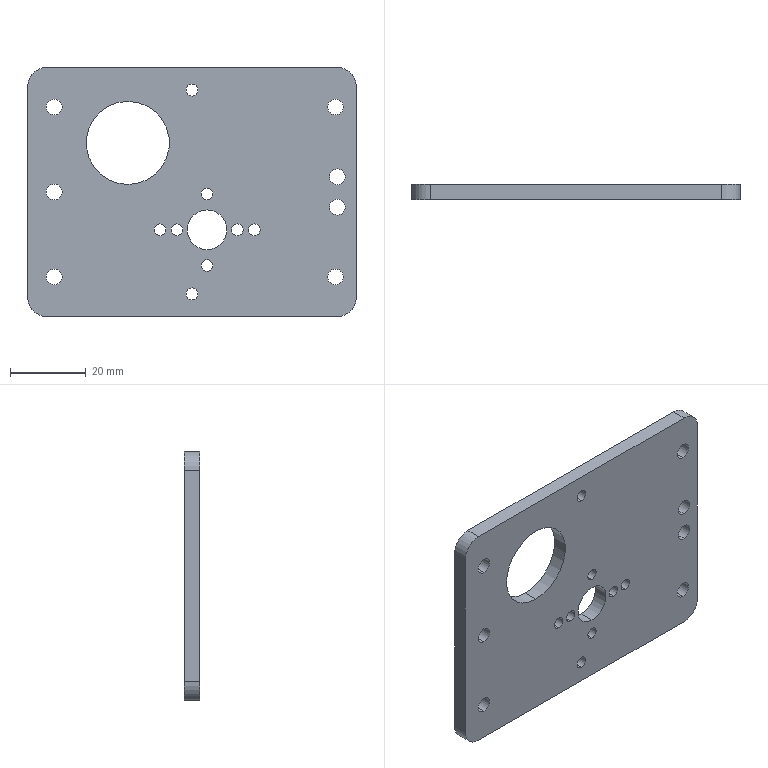Part | SolidWorks | features BaseBody 1 | 1 solid | 44 faces | box 87 x 4 x 66 mm | volume 20382 mm3 | cylinder 38 | plane 6 | commonest cylinder face diameters 4.2 x14 3.1 x12 3.2 x4 10 x4 10.5 x2 22 x2
STEP:
#1=CARTESIAN_POINT('',(38.5,4.,6.1));
#2=VERTEX_POINT('',#1);
#3=CARTESIAN_POINT('',(38.5,4.,1.9));
#4=VERTEX_POINT('',#3);
#5=CARTESIAN_POINT('',(38.5,4.,4.));
#6=DIRECTION('',(0.,-1.,0.));
#7=DIRECTION('',(0.,0.,-1.));
#8=AXIS2_PLACEMENT_3D('',#5,#6,#7);
#9=CIRCLE('',#8,2.1);
#10=EDGE_CURVE('',#2,#4,#9,.T.);
#11=ORIENTED_EDGE('',*,*,#10,.F.);
#12=CARTESIAN_POINT('',(38.5,0.,6.1));
#13=VERTEX_POINT('',#12);
#14=CARTESIAN_POINT('',(38.5,4.,6.1));
#15=DIRECTION('',(0.,-1.,0.));
#16=VECTOR('',#15,1000.);
#17=LINE('',#14,#16);
#18=EDGE_CURVE('',#2,#13,#17,.T.);
#19=ORIENTED_EDGE('',*,*,#18,.T.);
#20=CARTESIAN_POINT('',(38.5,0.,1.9));
#21=VERTEX_POINT('',#20);
#22=CARTESIAN_POINT('',(38.5,0.,4.));
#23=DIRECTION('',(0.,-1.,0.));
#24=DIRECTION('',(0.,0.,-1.));
#25=AXIS2_PLACEMENT_3D('',#22,#23,#24);
#26=CIRCLE('',#25,2.1);
#27=EDGE_CURVE('',#13,#21,#26,.T.);
#28=ORIENTED_EDGE('',*,*,#27,.T.);
#29=CARTESIAN_POINT('',(38.5,4.,1.9));
#30=DIRECTION('',(0.,-1.,0.));
#31=VECTOR('',#30,1000.);
#32=LINE('',#29,#31);
#33=EDGE_CURVE('',#4,#21,#32,.T.);
#34=ORIENTED_EDGE('',*,*,#33,.F.);
#35=EDGE_LOOP('',(#11,#19,#28,#34));
#36=FACE_OUTER_BOUND('',#35,.T.);
#37=CARTESIAN_POINT('',(38.5,4.,4.));
#38=DIRECTION('',(0.,-1.,0.));
#39=DIRECTION('',(0.,0.,-1.));
#40=AXIS2_PLACEMENT_3D('',#37,#38,#39);
#41=CYLINDRICAL_SURFACE('',#40,2.1);
#42=ADVANCED_FACE('',(#36),#41,.F.);
#43=CARTESIAN_POINT('',(38.5,4.,-1.9));
#44=VERTEX_POINT('',#43);
#45=CARTESIAN_POINT('',(38.5,4.,-6.1));
#46=VERTEX_POINT('',#45);
#47=CARTESIAN_POINT('',(38.5,4.,-4.));
#48=DIRECTION('',(0.,-1.,0.));
#49=DIRECTION('',(0.,0.,-1.));
#50=AXIS2_PLACEMENT_3D('',#47,#48,#49);
#51=CIRCLE('',#50,2.1);
#52=EDGE_CURVE('',#44,#46,#51,.T.);
#53=ORIENTED_EDGE('',*,*,#52,.F.);
#54=CARTESIAN_POINT('',(38.5,0.,-1.9));
#55=VERTEX_POINT('',#54);
#56=CARTESIAN_POINT('',(38.5,4.,-1.9));
#57=DIRECTION('',(0.,-1.,0.));
#58=VECTOR('',#57,1000.);
#59=LINE('',#56,#58);
#60=EDGE_CURVE('',#44,#55,#59,.T.);
#61=ORIENTED_EDGE('',*,*,#60,.T.);
#62=CARTESIAN_POINT('',(38.5,0.,-6.1));
#63=VERTEX_POINT('',#62);
#64=CARTESIAN_POINT('',(38.5,0.,-4.));
#65=DIRECTION('',(0.,-1.,0.));
#66=DIRECTION('',(0.,0.,-1.));
#67=AXIS2_PLACEMENT_3D('',#64,#65,#66);
#68=CIRCLE('',#67,2.1);
#69=EDGE_CURVE('',#55,#63,#68,.T.);
#70=ORIENTED_EDGE('',*,*,#69,.T.);
#71=CARTESIAN_POINT('',(38.5,4.,-6.1));
#72=DIRECTION('',(0.,-1.,0.));
#73=VECTOR('',#72,1000.);
#74=LINE('',#71,#73);
#75=EDGE_CURVE('',#46,#63,#74,.T.);
#76=ORIENTED_EDGE('',*,*,#75,.F.);
#77=EDGE_LOOP('',(#53,#61,#70,#76));
#78=FACE_OUTER_BOUND('',#77,.T.);
#79=CARTESIAN_POINT('',(38.5,4.,-4.));
#80=DIRECTION('',(0.,-1.,0.));
#81=DIRECTION('',(0.,0.,-1.));
#82=AXIS2_PLACEMENT_3D('',#79,#80,#81);
#83=CYLINDRICAL_SURFACE('',#82,2.1);
#84=ADVANCED_FACE('',(#78),#83,.F.);
#85=CARTESIAN_POINT('',(0.,4.,28.6));
#86=VERTEX_POINT('',#85);
#87=CARTESIAN_POINT('',(0.,4.,25.4));
#88=VERTEX_POINT('',#87);
#89=CARTESIAN_POINT('',(0.,4.,27.));
#90=DIRECTION('',(0.,-1.,0.));
#91=DIRECTION('',(0.,0.,-1.));
#92=AXIS2_PLACEMENT_3D('',#89,#90,#91);
#93=CIRCLE('',#92,1.6);
#94=EDGE_CURVE('',#86,#88,#93,.T.);
#95=ORIENTED_EDGE('',*,*,#94,.F.);
#96=CARTESIAN_POINT('',(0.,0.,28.6));
#97=VERTEX_POINT('',#96);
#98=CARTESIAN_POINT('',(0.,4.,28.6));
#99=DIRECTION('',(0.,-1.,0.));
#100=VECTOR('',#99,1000.);
#101=LINE('',#98,#100);
#102=EDGE_CURVE('',#86,#97,#101,.T.);
#103=ORIENTED_EDGE('',*,*,#102,.T.);
#104=CARTESIAN_POINT('',(0.,0.,25.4));
#105=VERTEX_POINT('',#104);
#106=CARTESIAN_POINT('',(0.,0.,27.));
#107=DIRECTION('',(0.,-1.,0.));
#108=DIRECTION('',(0.,0.,-1.));
#109=AXIS2_PLACEMENT_3D('',#106,#107,#108);
#110=CIRCLE('',#109,1.6);
#111=EDGE_CURVE('',#97,#105,#110,.T.);
#112=ORIENTED_EDGE('',*,*,#111,.T.);
#113=CARTESIAN_POINT('',(0.,4.,25.4));
#114=DIRECTION('',(0.,-1.,0.));
#115=VECTOR('',#114,1000.);
#116=LINE('',#113,#115);
#117=EDGE_CURVE('',#88,#105,#116,.T.);
#118=ORIENTED_EDGE('',*,*,#117,.F.);
#119=EDGE_LOOP('',(#95,#103,#112,#118));
#120=FACE_OUTER_BOUND('',#119,.T.);
#121=CARTESIAN_POINT('',(0.,4.,27.));
#122=DIRECTION('',(0.,-1.,0.));
#123=DIRECTION('',(0.,0.,-1.));
#124=AXIS2_PLACEMENT_3D('',#121,#122,#123);
#125=CYLINDRICAL_SURFACE('',#124,1.6);
#126=ADVANCED_FACE('',(#120),#125,.F.);
#127=CARTESIAN_POINT('',(38.,4.,-20.4));
#128=VERTEX_POINT('',#127);
#129=CARTESIAN_POINT('',(38.,4.,-24.6));
#130=VERTEX_POINT('',#129);
#131=CARTESIAN_POINT('',(38.,4.,-22.5));
#132=DIRECTION('',(0.,-1.,0.));
#133=DIRECTION('',(0.,0.,-1.));
#134=AXIS2_PLACEMENT_3D('',#131,#132,#133);
#135=CIRCLE('',#134,2.1);
#136=EDGE_CURVE('',#128,#130,#135,.T.);
#137=ORIENTED_EDGE('',*,*,#136,.F.);
#138=CARTESIAN_POINT('',(38.,0.,-20.4));
#139=VERTEX_POINT('',#138);
#140=CARTESIAN_POINT('',(38.,4.,-20.4));
#141=DIRECTION('',(0.,-1.,0.));
#142=VECTOR('',#141,1000.);
#143=LINE('',#140,#142);
#144=EDGE_CURVE('',#128,#139,#143,.T.);
#145=ORIENTED_EDGE('',*,*,#144,.T.);
#146=CARTESIAN_POINT('',(38.,0.,-24.6));
#147=VERTEX_POINT('',#146);
#148=CARTESIAN_POINT('',(38.,0.,-22.5));
#149=DIRECTION('',(0.,-1.,0.));
#150=DIRECTION('',(0.,0.,-1.));
#151=AXIS2_PLACEMENT_3D('',#148,#149,#150);
#152=CIRCLE('',#151,2.1);
#153=EDGE_CURVE('',#139,#147,#152,.T.);
#154=ORIENTED_EDGE('',*,*,#153,.T.);
#155=CARTESIAN_POINT('',(38.,4.,-24.6));
#156=DIRECTION('',(0.,-1.,0.));
#157=VECTOR('',#156,1000.);
#158=LINE('',#155,#157);
#159=EDGE_CURVE('',#130,#147,#158,.T.);
#160=ORIENTED_EDGE('',*,*,#159,.F.);
#161=EDGE_LOOP('',(#137,#145,#154,#160));
#162=FACE_OUTER_BOUND('',#161,.T.);
#163=CARTESIAN_POINT('',(38.,4.,-22.5));
#164=DIRECTION('',(0.,-1.,0.));
#165=DIRECTION('',(0.,0.,-1.));
#166=AXIS2_PLACEMENT_3D('',#163,#164,#165);
#167=CYLINDRICAL_SURFACE('',#166,2.1);
#168=ADVANCED_FACE('',(#162),#167,.F.);
#169=CARTESIAN_POINT('',(38.,4.,24.6));
#170=VERTEX_POINT('',#169);
#171=CARTESIAN_POINT('',(38.,4.,20.4));
#172=VERTEX_POINT('',#171);
#173=CARTESIAN_POINT('',(38.,4.,22.5));
#174=DIRECTION('',(0.,-1.,0.));
#175=DIRECTION('',(0.,0.,-1.));
#176=AXIS2_PLACEMENT_3D('',#173,#174,#175);
#177=CIRCLE('',#176,2.1);
#178=EDGE_CURVE('',#170,#172,#177,.T.);
#179=ORIENTED_EDGE('',*,*,#178,.F.);
#180=CARTESIAN_POINT('',(38.,0.,24.6));
#181=VERTEX_POINT('',#180);
#182=CARTESIAN_POINT('',(38.,4.,24.6));
#183=DIRECTION('',(0.,-1.,0.));
#184=VECTOR('',#183,1000.);
#185=LINE('',#182,#184);
#186=EDGE_CURVE('',#170,#181,#185,.T.);
#187=ORIENTED_EDGE('',*,*,#186,.T.);
#188=CARTESIAN_POINT('',(38.,0.,20.4));
#189=VERTEX_POINT('',#188);
#190=CARTESIAN_POINT('',(38.,0.,22.5));
#191=DIRECTION('',(0.,-1.,0.));
#192=DIRECTION('',(0.,0.,-1.));
#193=AXIS2_PLACEMENT_3D('',#190,#191,#192);
#194=CIRCLE('',#193,2.1);
#195=EDGE_CURVE('',#181,#189,#194,.T.);
#196=ORIENTED_EDGE('',*,*,#195,.T.);
#197=CARTESIAN_POINT('',(38.,4.,20.4));
#198=DIRECTION('',(0.,-1.,0.));
#199=VECTOR('',#198,1000.);
#200=LINE('',#197,#199);
#201=EDGE_CURVE('',#172,#189,#200,.T.);
#202=ORIENTED_EDGE('',*,*,#201,.F.);
#203=EDGE_LOOP('',(#179,#187,#196,#202));
#204=FACE_OUTER_BOUND('',#203,.T.);
#205=CARTESIAN_POINT('',(38.,4.,22.5));
#206=DIRECTION('',(0.,-1.,0.));
#207=DIRECTION('',(0.,0.,-1.));
#208=AXIS2_PLACEMENT_3D('',#205,#206,#207);
#209=CYLINDRICAL_SURFACE('',#208,2.1);
#210=ADVANCED_FACE('',(#204),#209,.F.);
#211=CARTESIAN_POINT('',(-36.5,4.,24.6));
#212=VERTEX_POINT('',#211);
#213=CARTESIAN_POINT('',(-36.5,4.,20.4));
#214=VERTEX_POINT('',#213);
#215=CARTESIAN_POINT('',(-36.5,4.,22.5));
#216=DIRECTION('',(0.,-1.,0.));
#217=DIRECTION('',(0.,0.,-1.));
#218=AXIS2_PLACEMENT_3D('',#215,#216,#217);
#219=CIRCLE('',#218,2.1);
#220=EDGE_CURVE('',#212,#214,#219,.T.);
#221=ORIENTED_EDGE('',*,*,#220,.F.);
#222=CARTESIAN_POINT('',(-36.5,0.,24.6));
#223=VERTEX_POINT('',#222);
#224=CARTESIAN_POINT('',(-36.5,4.,24.6));
#225=DIRECTION('',(0.,-1.,0.));
#226=VECTOR('',#225,1000.);
#227=LINE('',#224,#226);
#228=EDGE_CURVE('',#212,#223,#227,.T.);
#229=ORIENTED_EDGE('',*,*,#228,.T.);
#230=CARTESIAN_POINT('',(-36.5,0.,20.4));
#231=VERTEX_POINT('',#230);
#232=CARTESIAN_POINT('',(-36.5,0.,22.5));
#233=DIRECTION('',(0.,-1.,0.));
#234=DIRECTION('',(0.,0.,-1.));
#235=AXIS2_PLACEMENT_3D('',#232,#233,#234);
#236=CIRCLE('',#235,2.1);
#237=EDGE_CURVE('',#223,#231,#236,.T.);
#238=ORIENTED_EDGE('',*,*,#237,.T.);
#239=CARTESIAN_POINT('',(-36.5,4.,20.4));
#240=DIRECTION('',(0.,-1.,0.));
#241=VECTOR('',#240,1000.);
#242=LINE('',#239,#241);
#243=EDGE_CURVE('',#214,#231,#242,.T.);
#244=ORIENTED_EDGE('',*,*,#243,.F.);
#245=EDGE_LOOP('',(#221,#229,#238,#244));
#246=FACE_OUTER_BOUND('',#245,.T.);
#247=CARTESIAN_POINT('',(-36.5,4.,22.5));
#248=DIRECTION('',(0.,-1.,0.));
#249=DIRECTION('',(0.,0.,-1.));
#250=AXIS2_PLACEMENT_3D('',#247,#248,#249);
#251=CYLINDRICAL_SURFACE('',#250,2.1);
#252=ADVANCED_FACE('',(#246),#251,.F.);
#253=CARTESIAN_POINT('',(-36.5,4.,2.1));
#254=VERTEX_POINT('',#253);
#255=CARTESIAN_POINT('',(-36.5,4.,-2.1));
#256=VERTEX_POINT('',#255);
#257=CARTESIAN_POINT('',(-36.5,4.,0.));
#258=DIRECTION('',(0.,-1.,0.));
#259=DIRECTION('',(0.,0.,-1.));
#260=AXIS2_PLACEMENT_3D('',#257,#258,#259);
#261=CIRCLE('',#260,2.1);
#262=EDGE_CURVE('',#254,#256,#261,.T.);
#263=ORIENTED_EDGE('',*,*,#262,.F.);
#264=CARTESIAN_POINT('',(-36.5,0.,2.1));
#265=VERTEX_POINT('',#264);
#266=CARTESIAN_POINT('',(-36.5,4.,2.1));
#267=DIRECTION('',(0.,-1.,0.));
#268=VECTOR('',#267,1000.);
#269=LINE('',#266,#268);
#270=EDGE_CURVE('',#254,#265,#269,.T.);
#271=ORIENTED_EDGE('',*,*,#270,.T.);
#272=CARTESIAN_POINT('',(-36.5,0.,-2.1));
#273=VERTEX_POINT('',#272);
#274=CARTESIAN_POINT('',(-36.5,0.,0.));
#275=DIRECTION('',(0.,-1.,0.));
#276=DIRECTION('',(0.,0.,-1.));
#277=AXIS2_PLACEMENT_3D('',#274,#275,#276);
#278=CIRCLE('',#277,2.1);
#279=EDGE_CURVE('',#265,#273,#278,.T.);
#280=ORIENTED_EDGE('',*,*,#279,.T.);
#281=CARTESIAN_POINT('',(-36.5,4.,-2.1));
#282=DIRECTION('',(0.,-1.,0.));
#283=VECTOR('',#282,1000.);
#284=LINE('',#281,#283);
#285=EDGE_CURVE('',#256,#273,#284,.T.);
#286=ORIENTED_EDGE('',*,*,#285,.F.);
#287=EDGE_LOOP('',(#263,#271,#280,#286));
#288=FACE_OUTER_BOUND('',#287,.T.);
#289=CARTESIAN_POINT('',(-36.5,4.,0.));
#290=DIRECTION('',(0.,-1.,0.));
#291=DIRECTION('',(0.,0.,-1.));
#292=AXIS2_PLACEMENT_3D('',#289,#290,#291);
#293=CYLINDRICAL_SURFACE('',#292,2.1);
#294=ADVANCED_FACE('',(#288),#293,.F.);
#295=CARTESIAN_POINT('',(-36.5,4.,-20.4));
#296=VERTEX_POINT('',#295);
#297=CARTESIAN_POINT('',(-36.5,4.,-24.6));
#298=VERTEX_POINT('',#297);
#299=CARTESIAN_POINT('',(-36.5,4.,-22.5));
#300=DIRECTION('',(0.,-1.,0.));
#301=DIRECTION('',(0.,0.,-1.));
#302=AXIS2_PLACEMENT_3D('',#299,#300,#301);
#303=CIRCLE('',#302,2.1);
#304=EDGE_CURVE('',#296,#298,#303,.T.);
#305=ORIENTED_EDGE('',*,*,#304,.F.);
#306=CARTESIAN_POINT('',(-36.5,0.,-20.4));
#307=VERTEX_POINT('',#306);
#308=CARTESIAN_POINT('',(-36.5,4.,-20.4));
#309=DIRECTION('',(0.,-1.,0.));
#310=VECTOR('',#309,1000.);
#311=LINE('',#308,#310);
#312=EDGE_CURVE('',#296,#307,#311,.T.);
#313=ORIENTED_EDGE('',*,*,#312,.T.);
#314=CARTESIAN_POINT('',(-36.5,0.,-24.6));
#315=VERTEX_POINT('',#314);
#316=CARTESIAN_POINT('',(-36.5,0.,-22.5));
#317=DIRECTION('',(0.,-1.,0.));
#318=DIRECTION('',(0.,0.,-1.));
#319=AXIS2_PLACEMENT_3D('',#316,#317,#318);
#320=CIRCLE('',#319,2.1);
#321=EDGE_CURVE('',#307,#315,#320,.T.);
#322=ORIENTED_EDGE('',*,*,#321,.T.);
#323=CARTESIAN_POINT('',(-36.5,4.,-24.6));
#324=DIRECTION('',(0.,-1.,0.));
#325=VECTOR('',#324,1000.);
#326=LINE('',#323,#325);
#327=EDGE_CURVE('',#298,#315,#326,.T.);
#328=ORIENTED_EDGE('',*,*,#327,.F.);
#329=EDGE_LOOP('',(#305,#313,#322,#328));
#330=FACE_OUTER_BOUND('',#329,.T.);
#331=CARTESIAN_POINT('',(-36.5,4.,-22.5));
#332=DIRECTION('',(0.,-1.,0.));
#333=DIRECTION('',(0.,0.,-1.));
#334=AXIS2_PLACEMENT_3D('',#331,#332,#333);
#335=CYLINDRICAL_SURFACE('',#334,2.1);
#336=ADVANCED_FACE('',(#330),#335,.F.);
#337=CARTESIAN_POINT('',(0.,4.,-25.4));
#338=VERTEX_POINT('',#337);
#339=CARTESIAN_POINT('',(0.,4.,-28.6));
#340=VERTEX_POINT('',#339);
#341=CARTESIAN_POINT('',(0.,4.,-27.));
#342=DIRECTION('',(0.,-1.,0.));
#343=DIRECTION('',(0.,0.,-1.));
#344=AXIS2_PLACEMENT_3D('',#341,#342,#343);
#345=CIRCLE('',#344,1.6);
#346=EDGE_CURVE('',#338,#340,#345,.T.);
#347=ORIENTED_EDGE('',*,*,#346,.F.);
#348=CARTESIAN_POINT('',(0.,0.,-25.4));
#349=VERTEX_POINT('',#348);
#350=CARTESIAN_POINT('',(0.,4.,-25.4));
#351=DIRECTION('',(0.,-1.,0.));
#352=VECTOR('',#351,1000.);
#353=LINE('',#350,#352);
#354=EDGE_CURVE('',#338,#349,#353,.T.);
#355=ORIENTED_EDGE('',*,*,#354,.T.);
#356=CARTESIAN_POINT('',(0.,0.,-28.6));
#357=VERTEX_POINT('',#356);
#358=CARTESIAN_POINT('',(0.,0.,-27.));
#359=DIRECTION('',(0.,-1.,0.));
#360=DIRECTION('',(0.,0.,-1.));
#361=AXIS2_PLACEMENT_3D('',#358,#359,#360);
#362=CIRCLE('',#361,1.6);
#363=EDGE_CURVE('',#349,#357,#362,.T.);
#364=ORIENTED_EDGE('',*,*,#363,.T.);
#365=CARTESIAN_POINT('',(0.,4.,-28.6));
#366=DIRECTION('',(0.,-1.,0.));
#367=VECTOR('',#366,1000.);
#368=LINE('',#365,#367);
#369=EDGE_CURVE('',#340,#357,#368,.T.);
#370=ORIENTED_EDGE('',*,*,#369,.F.);
#371=EDGE_LOOP('',(#347,#355,#364,#370));
#372=FACE_OUTER_BOUND('',#371,.T.);
#373=CARTESIAN_POINT('',(0.,4.,-27.));
#374=DIRECTION('',(0.,-1.,0.));
#375=DIRECTION('',(0.,0.,-1.));
#376=AXIS2_PLACEMENT_3D('',#373,#374,#375);
#377=CYLINDRICAL_SURFACE('',#376,1.6);
#378=ADVANCED_FACE('',(#372),#377,.F.);
#379=CARTESIAN_POINT('',(4.,4.,-4.75));
#380=VERTEX_POINT('',#379);
#381=CARTESIAN_POINT('',(4.,4.,-15.25));
#382=VERTEX_POINT('',#381);
#383=CARTESIAN_POINT('',(4.,4.,-10.));
#384=DIRECTION('',(0.,-1.,0.));
#385=DIRECTION('',(0.,0.,-1.));
#386=AXIS2_PLACEMENT_3D('',#383,#384,#385);
#387=CIRCLE('',#386,5.25);
#388=EDGE_CURVE('',#380,#382,#387,.T.);
#389=ORIENTED_EDGE('',*,*,#388,.F.);
#390=CARTESIAN_POINT('',(4.,0.,-4.75));
#391=VERTEX_POINT('',#390);
#392=CARTESIAN_POINT('',(4.,4.,-4.75));
#393=DIRECTION('',(0.,-1.,0.));
#394=VECTOR('',#393,1000.);
#395=LINE('',#392,#394);
#396=EDGE_CURVE('',#380,#391,#395,.T.);
#397=ORIENTED_EDGE('',*,*,#396,.T.);
#398=CARTESIAN_POINT('',(4.,0.,-15.25));
#399=VERTEX_POINT('',#398);
#400=CARTESIAN_POINT('',(4.,0.,-10.));
#401=DIRECTION('',(0.,-1.,0.));
#402=DIRECTION('',(0.,0.,-1.));
#403=AXIS2_PLACEMENT_3D('',#400,#401,#402);
#404=CIRCLE('',#403,5.25);
#405=EDGE_CURVE('',#391,#399,#404,.T.);
#406=ORIENTED_EDGE('',*,*,#405,.T.);
#407=CARTESIAN_POINT('',(4.,4.,-15.25));
#408=DIRECTION('',(0.,-1.,0.));
#409=VECTOR('',#408,1000.);
#410=LINE('',#407,#409);
#411=EDGE_CURVE('',#382,#399,#410,.T.);
#412=ORIENTED_EDGE('',*,*,#411,.F.);
#413=EDGE_LOOP('',(#389,#397,#406,#412));
#414=FACE_OUTER_BOUND('',#413,.T.);
#415=CARTESIAN_POINT('',(4.,4.,-10.));
#416=DIRECTION('',(0.,-1.,0.));
#417=DIRECTION('',(0.,0.,-1.));
#418=AXIS2_PLACEMENT_3D('',#415,#416,#417);
#419=CYLINDRICAL_SURFACE('',#418,5.25);
#420=ADVANCED_FACE('',(#414),#419,.F.);
#421=CARTESIAN_POINT('',(-4.,4.,-8.45));
#422=VERTEX_POINT('',#421);
#423=CARTESIAN_POINT('',(-4.,4.,-11.55));
#424=VERTEX_POINT('',#423);
#425=CARTESIAN_POINT('',(-4.,4.,-10.));
#426=DIRECTION('',(0.,-1.,0.));
#427=DIRECTION('',(0.,0.,-1.));
#428=AXIS2_PLACEMENT_3D('',#425,#426,#427);
#429=CIRCLE('',#428,1.55);
#430=EDGE_CURVE('',#422,#424,#429,.T.);
#431=ORIENTED_EDGE('',*,*,#430,.F.);
#432=CARTESIAN_POINT('',(-4.,0.,-8.45));
#433=VERTEX_POINT('',#432);
#434=CARTESIAN_POINT('',(-4.,4.,-8.45));
#435=DIRECTION('',(0.,-1.,0.));
#436=VECTOR('',#435,1000.);
#437=LINE('',#434,#436);
#438=EDGE_CURVE('',#422,#433,#437,.T.);
#439=ORIENTED_EDGE('',*,*,#438,.T.);
#440=CARTESIAN_POINT('',(-4.,0.,-11.55));
#441=VERTEX_POINT('',#440);
#442=CARTESIAN_POINT('',(-4.,0.,-10.));
#443=DIRECTION('',(0.,-1.,0.));
#444=DIRECTION('',(0.,0.,-1.));
#445=AXIS2_PLACEMENT_3D('',#442,#443,#444);
#446=CIRCLE('',#445,1.55);
#447=EDGE_CURVE('',#433,#441,#446,.T.);
#448=ORIENTED_EDGE('',*,*,#447,.T.);
#449=CARTESIAN_POINT('',(-4.,4.,-11.55));
#450=DIRECTION('',(0.,-1.,0.));
#451=VECTOR('',#450,1000.);
#452=LINE('',#449,#451);
#453=EDGE_CURVE('',#424,#441,#452,.T.);
#454=ORIENTED_EDGE('',*,*,#453,.F.);
#455=EDGE_LOOP('',(#431,#439,#448,#454));
#456=FACE_OUTER_BOUND('',#455,.T.);
#457=CARTESIAN_POINT('',(-4.,4.,-10.));
#458=DIRECTION('',(0.,-1.,0.));
#459=DIRECTION('',(0.,0.,-1.));
#460=AXIS2_PLACEMENT_3D('',#457,#458,#459);
#461=CYLINDRICAL_SURFACE('',#460,1.55);
#462=ADVANCED_FACE('',(#456),#461,.F.);
#463=CARTESIAN_POINT('',(4.,4.,1.05));
#464=VERTEX_POINT('',#463);
#465=CARTESIAN_POINT('',(4.,4.,-2.05));
#466=VERTEX_POINT('',#465);
#467=CARTESIAN_POINT('',(4.,4.,-0.5));
#468=DIRECTION('',(0.,-1.,0.));
#469=DIRECTION('',(0.,0.,-1.));
#470=AXIS2_PLACEMENT_3D('',#467,#468,#469);
#471=CIRCLE('',#470,1.55);
#472=EDGE_CURVE('',#464,#466,#471,.T.);
#473=ORIENTED_EDGE('',*,*,#472,.F.);
#474=CARTESIAN_POINT('',(4.,0.,1.05));
#475=VERTEX_POINT('',#474);
#476=CARTESIAN_POINT('',(4.,4.,1.05));
#477=DIRECTION('',(0.,-1.,0.));
#478=VECTOR('',#477,1000.);
#479=LINE('',#476,#478);
#480=EDGE_CURVE('',#464,#475,#479,.T.);
#481=ORIENTED_EDGE('',*,*,#480,.T.);
#482=CARTESIAN_POINT('',(4.,0.,-2.05));
#483=VERTEX_POINT('',#482);
#484=CARTESIAN_POINT('',(4.,0.,-0.5));
#485=DIRECTION('',(0.,-1.,0.));
#486=DIRECTION('',(0.,0.,-1.));
#487=AXIS2_PLACEMENT_3D('',#484,#485,#486);
#488=CIRCLE('',#487,1.55);
#489=EDGE_CURVE('',#475,#483,#488,.T.);
#490=ORIENTED_EDGE('',*,*,#489,.T.);
#491=CARTESIAN_POINT('',(4.,4.,-2.05));
#492=DIRECTION('',(0.,-1.,0.));
#493=VECTOR('',#492,1000.);
#494=LINE('',#491,#493);
#495=EDGE_CURVE('',#466,#483,#494,.T.);
#496=ORIENTED_EDGE('',*,*,#495,.F.);
#497=EDGE_LOOP('',(#473,#481,#490,#496));
#498=FACE_OUTER_BOUND('',#497,.T.);
#499=CARTESIAN_POINT('',(4.,4.,-0.5));
#500=DIRECTION('',(0.,-1.,0.));
#501=DIRECTION('',(0.,0.,-1.));
#502=AXIS2_PLACEMENT_3D('',#499,#500,#501);
#503=CYLINDRICAL_SURFACE('',#502,1.55);
#504=ADVANCED_FACE('',(#498),#503,.F.);
#505=CARTESIAN_POINT('',(4.,4.,-17.95));
#506=VERTEX_POINT('',#505);
#507=CARTESIAN_POINT('',(4.,4.,-21.05));
#508=VERTEX_POINT('',#507);
#509=CARTESIAN_POINT('',(4.,4.,-19.5));
#510=DIRECTION('',(0.,-1.,0.));
#511=DIRECTION('',(0.,0.,-1.));
#512=AXIS2_PLACEMENT_3D('',#509,#510,#511);
#513=CIRCLE('',#512,1.55);
#514=EDGE_CURVE('',#506,#508,#513,.T.);
#515=ORIENTED_EDGE('',*,*,#514,.F.);
#516=CARTESIAN_POINT('',(4.,0.,-17.95));
#517=VERTEX_POINT('',#516);
#518=CARTESIAN_POINT('',(4.,4.,-17.95));
#519=DIRECTION('',(0.,-1.,0.));
#520=VECTOR('',#519,1000.);
#521=LINE('',#518,#520);
#522=EDGE_CURVE('',#506,#517,#521,.T.);
#523=ORIENTED_EDGE('',*,*,#522,.T.);
#524=CARTESIAN_POINT('',(4.,0.,-21.05));
#525=VERTEX_POINT('',#524);
#526=CARTESIAN_POINT('',(4.,0.,-19.5));
#527=DIRECTION('',(0.,-1.,0.));
#528=DIRECTION('',(0.,0.,-1.));
#529=AXIS2_PLACEMENT_3D('',#526,#527,#528);
#530=CIRCLE('',#529,1.55);
#531=EDGE_CURVE('',#517,#525,#530,.T.);
#532=ORIENTED_EDGE('',*,*,#531,.T.);
#533=CARTESIAN_POINT('',(4.,4.,-21.05));
#534=DIRECTION('',(0.,-1.,0.));
#535=VECTOR('',#534,1000.);
#536=LINE('',#533,#535);
#537=EDGE_CURVE('',#508,#525,#536,.T.);
#538=ORIENTED_EDGE('',*,*,#537,.F.);
#539=EDGE_LOOP('',(#515,#523,#532,#538));
#540=FACE_OUTER_BOUND('',#539,.T.);
#541=CARTESIAN_POINT('',(4.,4.,-19.5));
#542=DIRECTION('',(0.,-1.,0.));
#543=DIRECTION('',(0.,0.,-1.));
#544=AXIS2_PLACEMENT_3D('',#541,#542,#543);
#545=CYLINDRICAL_SURFACE('',#544,1.55);
#546=ADVANCED_FACE('',(#540),#545,.F.);
#547=CARTESIAN_POINT('',(16.5,4.,-8.45));
#548=VERTEX_POINT('',#547);
#549=CARTESIAN_POINT('',(16.5,4.,-11.55));
#550=VERTEX_POINT('',#549);
#551=CARTESIAN_POINT('',(16.5,4.,-10.));
#552=DIRECTION('',(0.,-1.,0.));
#553=DIRECTION('',(0.,0.,-1.));
#554=AXIS2_PLACEMENT_3D('',#551,#552,#553);
#555=CIRCLE('',#554,1.55);
#556=EDGE_CURVE('',#548,#550,#555,.T.);
#557=ORIENTED_EDGE('',*,*,#556,.F.);
#558=CARTESIAN_POINT('',(16.5,0.,-8.45));
#559=VERTEX_POINT('',#558);
#560=CARTESIAN_POINT('',(16.5,4.,-8.45));
#561=DIRECTION('',(0.,-1.,0.));
#562=VECTOR('',#561,1000.);
#563=LINE('',#560,#562);
#564=EDGE_CURVE('',#548,#559,#563,.T.);
#565=ORIENTED_EDGE('',*,*,#564,.T.);
#566=CARTESIAN_POINT('',(16.5,0.,-11.55));
#567=VERTEX_POINT('',#566);
#568=CARTESIAN_POINT('',(16.5,0.,-10.));
#569=DIRECTION('',(0.,-1.,0.));
#570=DIRECTION('',(0.,0.,-1.));
#571=AXIS2_PLACEMENT_3D('',#568,#569,#570);
#572=CIRCLE('',#571,1.55);
#573=EDGE_CURVE('',#559,#567,#572,.T.);
#574=ORIENTED_EDGE('',*,*,#573,.T.);
#575=CARTESIAN_POINT('',(16.5,4.,-11.55));
#576=DIRECTION('',(0.,-1.,0.));
#577=VECTOR('',#576,1000.);
#578=LINE('',#575,#577);
#579=EDGE_CURVE('',#550,#567,#578,.T.);
#580=ORIENTED_EDGE('',*,*,#579,.F.);
#581=EDGE_LOOP('',(#557,#565,#574,#580));
#582=FACE_OUTER_BOUND('',#581,.T.);
#583=CARTESIAN_POINT('',(16.5,4.,-10.));
#584=DIRECTION('',(0.,-1.,0.));
#585=DIRECTION('',(0.,0.,-1.));
#586=AXIS2_PLACEMENT_3D('',#583,#584,#585);
#587=CYLINDRICAL_SURFACE('',#586,1.55);
#588=ADVANCED_FACE('',(#582),#587,.F.);
#589=CARTESIAN_POINT('',(12.,4.,-8.45));
#590=VERTEX_POINT('',#589);
#591=CARTESIAN_POINT('',(12.,4.,-11.55));
#592=VERTEX_POINT('',#591);
#593=CARTESIAN_POINT('',(12.,4.,-10.));
#594=DIRECTION('',(0.,-1.,0.));
#595=DIRECTION('',(0.,0.,-1.));
#596=AXIS2_PLACEMENT_3D('',#593,#594,#595);
#597=CIRCLE('',#596,1.55);
#598=EDGE_CURVE('',#590,#592,#597,.T.);
#599=ORIENTED_EDGE('',*,*,#598,.F.);
#600=CARTESIAN_POINT('',(12.,0.,-8.45));
#601=VERTEX_POINT('',#600);
#602=CARTESIAN_POINT('',(12.,4.,-8.45));
#603=DIRECTION('',(0.,-1.,0.));
#604=VECTOR('',#603,1000.);
#605=LINE('',#602,#604);
#606=EDGE_CURVE('',#590,#601,#605,.T.);
#607=ORIENTED_EDGE('',*,*,#606,.T.);
#608=CARTESIAN_POINT('',(12.,0.,-11.55));
#609=VERTEX_POINT('',#608);
#610=CARTESIAN_POINT('',(12.,0.,-10.));
#611=DIRECTION('',(0.,-1.,0.));
#612=DIRECTION('',(0.,0.,-1.));
#613=AXIS2_PLACEMENT_3D('',#610,#611,#612);
#614=CIRCLE('',#613,1.55);
#615=EDGE_CURVE('',#601,#609,#614,.T.);
#616=ORIENTED_EDGE('',*,*,#615,.T.);
#617=CARTESIAN_POINT('',(12.,4.,-11.55));
#618=DIRECTION('',(0.,-1.,0.));
#619=VECTOR('',#618,1000.);
#620=LINE('',#617,#619);
#621=EDGE_CURVE('',#592,#609,#620,.T.);
#622=ORIENTED_EDGE('',*,*,#621,.F.);
#623=EDGE_LOOP('',(#599,#607,#616,#622));
#624=FACE_OUTER_BOUND('',#623,.T.);
#625=CARTESIAN_POINT('',(12.,4.,-10.));
#626=DIRECTION('',(0.,-1.,0.));
#627=DIRECTION('',(0.,0.,-1.));
#628=AXIS2_PLACEMENT_3D('',#625,#626,#627);
#629=CYLINDRICAL_SURFACE('',#628,1.55);
#630=ADVANCED_FACE('',(#624),#629,.F.);
#631=CARTESIAN_POINT('',(-8.5,4.,-8.45));
#632=VERTEX_POINT('',#631);
#633=CARTESIAN_POINT('',(-8.5,4.,-11.55));
#634=VERTEX_POINT('',#633);
#635=CARTESIAN_POINT('',(-8.5,4.,-10.));
#636=DIRECTION('',(0.,-1.,0.));
#637=DIRECTION('',(0.,0.,-1.));
#638=AXIS2_PLACEMENT_3D('',#635,#636,#637);
#639=CIRCLE('',#638,1.55);
#640=EDGE_CURVE('',#632,#634,#639,.T.);
#641=ORIENTED_EDGE('',*,*,#640,.F.);
#642=CARTESIAN_POINT('',(-8.5,0.,-8.45));
#643=VERTEX_POINT('',#642);
#644=CARTESIAN_POINT('',(-8.5,4.,-8.45));
#645=DIRECTION('',(0.,-1.,0.));
#646=VECTOR('',#645,1000.);
#647=LINE('',#644,#646);
#648=EDGE_CURVE('',#632,#643,#647,.T.);
#649=ORIENTED_EDGE('',*,*,#648,.T.);
#650=CARTESIAN_POINT('',(-8.5,0.,-11.55));
#651=VERTEX_POINT('',#650);
#652=CARTESIAN_POINT('',(-8.5,0.,-10.));
#653=DIRECTION('',(0.,-1.,0.));
#654=DIRECTION('',(0.,0.,-1.));
#655=AXIS2_PLACEMENT_3D('',#652,#653,#654);
#656=CIRCLE('',#655,1.55);
#657=EDGE_CURVE('',#643,#651,#656,.T.);
#658=ORIENTED_EDGE('',*,*,#657,.T.);
#659=CARTESIAN_POINT('',(-8.5,4.,-11.55));
#660=DIRECTION('',(0.,-1.,0.));
#661=VECTOR('',#660,1000.);
#662=LINE('',#659,#661);
#663=EDGE_CURVE('',#634,#651,#662,.T.);
#664=ORIENTED_EDGE('',*,*,#663,.F.);
#665=EDGE_LOOP('',(#641,#649,#658,#664));
#666=FACE_OUTER_BOUND('',#665,.T.);
#667=CARTESIAN_POINT('',(-8.5,4.,-10.));
#668=DIRECTION('',(0.,-1.,0.));
#669=DIRECTION('',(0.,0.,-1.));
#670=AXIS2_PLACEMENT_3D('',#667,#668,#669);
#671=CYLINDRICAL_SURFACE('',#670,1.55);
#672=ADVANCED_FACE('',(#666),#671,.F.);
#673=CARTESIAN_POINT('',(-17.,0.,24.));
#674=VERTEX_POINT('',#673);
#675=CARTESIAN_POINT('',(-17.,0.,2.));
#676=VERTEX_POINT('',#675);
#677=CARTESIAN_POINT('',(-17.,0.,13.));
#678=DIRECTION('',(0.,-1.,0.));
#679=DIRECTION('',(0.,0.,1.));
#680=AXIS2_PLACEMENT_3D('',#677,#678,#679);
#681=CIRCLE('',#680,11.);
#682=EDGE_CURVE('',#674,#676,#681,.T.);
#683=ORIENTED_EDGE('',*,*,#682,.T.);
#684=CARTESIAN_POINT('',(-17.,4.,2.));
#685=VERTEX_POINT('',#684);
#686=CARTESIAN_POINT('',(-17.,0.,2.));
#687=DIRECTION('',(0.,1.,0.));
#688=VECTOR('',#687,1000.);
#689=LINE('',#686,#688);
#690=EDGE_CURVE('',#676,#685,#689,.T.);
#691=ORIENTED_EDGE('',*,*,#690,.T.);
#692=CARTESIAN_POINT('',(-17.,4.,24.));
#693=VERTEX_POINT('',#692);
#694=CARTESIAN_POINT('',(-17.,4.,13.));
#695=DIRECTION('',(0.,-1.,0.));
#696=DIRECTION('',(0.,0.,1.));
#697=AXIS2_PLACEMENT_3D('',#694,#695,#696);
#698=CIRCLE('',#697,11.);
#699=EDGE_CURVE('',#693,#685,#698,.T.);
#700=ORIENTED_EDGE('',*,*,#699,.F.);
#701=CARTESIAN_POINT('',(-17.,0.,24.));
#702=DIRECTION('',(0.,1.,0.));
#703=VECTOR('',#702,1000.);
#704=LINE('',#701,#703);
#705=EDGE_CURVE('',#674,#693,#704,.T.);
#706=ORIENTED_EDGE('',*,*,#705,.F.);
#707=EDGE_LOOP('',(#683,#691,#700,#706));
#708=FACE_OUTER_BOUND('',#707,.T.);
#709=CARTESIAN_POINT('',(-17.,0.,13.));
#710=DIRECTION('',(0.,1.,0.));
#711=DIRECTION('',(0.,0.,1.));
#712=AXIS2_PLACEMENT_3D('',#709,#710,#711);
#713=CYLINDRICAL_SURFACE('',#712,11.);
#714=ADVANCED_FACE('',(#708),#713,.F.);
#715=CARTESIAN_POINT('',(38.5,0.,4.));
#716=DIRECTION('',(0.,-1.,0.));
#717=DIRECTION('',(0.,0.,-1.));
#718=AXIS2_PLACEMENT_3D('',#715,#716,#717);
#719=CIRCLE('',#718,2.1);
#720=EDGE_CURVE('',#21,#13,#719,.T.);
#721=ORIENTED_EDGE('',*,*,#720,.F.);
#722=ORIENTED_EDGE('',*,*,#27,.F.);
#723=EDGE_LOOP('',(#721,#722));
#724=FACE_BOUND('',#723,.T.);
#725=CARTESIAN_POINT('',(38.5,0.,-4.));
#726=DIRECTION('',(0.,-1.,0.));
#727=DIRECTION('',(0.,0.,-1.));
#728=AXIS2_PLACEMENT_3D('',#725,#726,#727);
#729=CIRCLE('',#728,2.1);
#730=EDGE_CURVE('',#63,#55,#729,.T.);
#731=ORIENTED_EDGE('',*,*,#730,.F.);
#732=ORIENTED_EDGE('',*,*,#69,.F.);
#733=EDGE_LOOP('',(#731,#732));
#734=FACE_BOUND('',#733,.T.);
#735=CARTESIAN_POINT('',(0.,0.,27.));
#736=DIRECTION('',(0.,-1.,0.));
#737=DIRECTION('',(0.,0.,-1.));
#738=AXIS2_PLACEMENT_3D('',#735,#736,#737);
#739=CIRCLE('',#738,1.6);
#740=EDGE_CURVE('',#105,#97,#739,.T.);
#741=ORIENTED_EDGE('',*,*,#740,.F.);
#742=ORIENTED_EDGE('',*,*,#111,.F.);
#743=EDGE_LOOP('',(#741,#742));
#744=FACE_BOUND('',#743,.T.);
#745=CARTESIAN_POINT('',(38.,0.,-22.5));
#746=DIRECTION('',(0.,-1.,0.));
#747=DIRECTION('',(0.,0.,-1.));
#748=AXIS2_PLACEMENT_3D('',#745,#746,#747);
#749=CIRCLE('',#748,2.1);
#750=EDGE_CURVE('',#147,#139,#749,.T.);
#751=ORIENTED_EDGE('',*,*,#750,.F.);
#752=ORIENTED_EDGE('',*,*,#153,.F.);
#753=EDGE_LOOP('',(#751,#752));
#754=FACE_BOUND('',#753,.T.);
#755=CARTESIAN_POINT('',(38.,0.,22.5));
#756=DIRECTION('',(0.,-1.,0.));
#757=DIRECTION('',(0.,0.,-1.));
#758=AXIS2_PLACEMENT_3D('',#755,#756,#757);
#759=CIRCLE('',#758,2.1);
#760=EDGE_CURVE('',#189,#181,#759,.T.);
#761=ORIENTED_EDGE('',*,*,#760,.F.);
#762=ORIENTED_EDGE('',*,*,#195,.F.);
#763=EDGE_LOOP('',(#761,#762));
#764=FACE_BOUND('',#763,.T.);
#765=CARTESIAN_POINT('',(-36.5,0.,22.5));
#766=DIRECTION('',(0.,-1.,0.));
#767=DIRECTION('',(0.,0.,-1.));
#768=AXIS2_PLACEMENT_3D('',#765,#766,#767);
#769=CIRCLE('',#768,2.1);
#770=EDGE_CURVE('',#231,#223,#769,.T.);
#771=ORIENTED_EDGE('',*,*,#770,.F.);
#772=ORIENTED_EDGE('',*,*,#237,.F.);
#773=EDGE_LOOP('',(#771,#772));
#774=FACE_BOUND('',#773,.T.);
#775=CARTESIAN_POINT('',(-36.5,0.,0.));
#776=DIRECTION('',(0.,-1.,0.));
#777=DIRECTION('',(0.,0.,-1.));
#778=AXIS2_PLACEMENT_3D('',#775,#776,#777);
#779=CIRCLE('',#778,2.1);
#780=EDGE_CURVE('',#273,#265,#779,.T.);
#781=ORIENTED_EDGE('',*,*,#780,.F.);
#782=ORIENTED_EDGE('',*,*,#279,.F.);
#783=EDGE_LOOP('',(#781,#782));
#784=FACE_BOUND('',#783,.T.);
#785=CARTESIAN_POINT('',(-36.5,0.,-22.5));
#786=DIRECTION('',(0.,-1.,0.));
#787=DIRECTION('',(0.,0.,-1.));
#788=AXIS2_PLACEMENT_3D('',#785,#786,#787);
#789=CIRCLE('',#788,2.1);
#790=EDGE_CURVE('',#315,#307,#789,.T.);
#791=ORIENTED_EDGE('',*,*,#790,.F.);
#792=ORIENTED_EDGE('',*,*,#321,.F.);
#793=EDGE_LOOP('',(#791,#792));
#794=FACE_BOUND('',#793,.T.);
#795=CARTESIAN_POINT('',(0.,0.,-27.));
#796=DIRECTION('',(0.,-1.,0.));
#797=DIRECTION('',(0.,0.,-1.));
#798=AXIS2_PLACEMENT_3D('',#795,#796,#797);
#799=CIRCLE('',#798,1.6);
#800=EDGE_CURVE('',#357,#349,#799,.T.);
#801=ORIENTED_EDGE('',*,*,#800,.F.);
#802=ORIENTED_EDGE('',*,*,#363,.F.);
#803=EDGE_LOOP('',(#801,#802));
#804=FACE_BOUND('',#803,.T.);
#805=CARTESIAN_POINT('',(38.5,0.,33.));
#806=VERTEX_POINT('',#805);
#807=CARTESIAN_POINT('',(43.5,0.,28.));
#808=VERTEX_POINT('',#807);
#809=CARTESIAN_POINT('',(38.5,0.,28.));
#810=DIRECTION('',(0.,1.,0.));
#811=DIRECTION('',(0.,0.,-1.));
#812=AXIS2_PLACEMENT_3D('',#809,#810,#811);
#813=CIRCLE('',#812,5.);
#814=EDGE_CURVE('',#806,#808,#813,.T.);
#815=ORIENTED_EDGE('',*,*,#814,.F.);
#816=CARTESIAN_POINT('',(-38.5,0.,33.));
#817=VERTEX_POINT('',#816);
#818=CARTESIAN_POINT('',(0.,0.,33.));
#819=DIRECTION('',(1.,0.,0.));
#820=VECTOR('',#819,1000.);
#821=LINE('',#818,#820);
#822=EDGE_CURVE('',#817,#806,#821,.T.);
#823=ORIENTED_EDGE('',*,*,#822,.F.);
#824=CARTESIAN_POINT('',(-43.5,0.,28.));
#825=VERTEX_POINT('',#824);
#826=CARTESIAN_POINT('',(-38.5,0.,28.));
#827=DIRECTION('',(0.,1.,0.));
#828=DIRECTION('',(0.,0.,-1.));
#829=AXIS2_PLACEMENT_3D('',#826,#827,#828);
#830=CIRCLE('',#829,5.);
#831=EDGE_CURVE('',#825,#817,#830,.T.);
#832=ORIENTED_EDGE('',*,*,#831,.F.);
#833=CARTESIAN_POINT('',(-43.5,0.,-28.));
#834=VERTEX_POINT('',#833);
#835=CARTESIAN_POINT('',(-43.5,0.,0.));
#836=DIRECTION('',(0.,0.,1.));
#837=VECTOR('',#836,1000.);
#838=LINE('',#835,#837);
#839=EDGE_CURVE('',#834,#825,#838,.T.);
#840=ORIENTED_EDGE('',*,*,#839,.F.);
#841=CARTESIAN_POINT('',(-38.5,0.,-33.));
#842=VERTEX_POINT('',#841);
#843=CARTESIAN_POINT('',(-38.5,0.,-28.));
#844=DIRECTION('',(0.,1.,0.));
#845=DIRECTION('',(0.,0.,-1.));
#846=AXIS2_PLACEMENT_3D('',#843,#844,#845);
#847=CIRCLE('',#846,5.);
#848=EDGE_CURVE('',#842,#834,#847,.T.);
#849=ORIENTED_EDGE('',*,*,#848,.F.);
#850=CARTESIAN_POINT('',(38.5,0.,-33.));
#851=VERTEX_POINT('',#850);
#852=CARTESIAN_POINT('',(0.,0.,-33.));
#853=DIRECTION('',(-1.,0.,0.));
#854=VECTOR('',#853,1000.);
#855=LINE('',#852,#854);
#856=EDGE_CURVE('',#851,#842,#855,.T.);
#857=ORIENTED_EDGE('',*,*,#856,.F.);
#858=CARTESIAN_POINT('',(43.5,0.,-28.));
#859=VERTEX_POINT('',#858);
#860=CARTESIAN_POINT('',(38.5,0.,-28.));
#861=DIRECTION('',(0.,1.,0.));
#862=DIRECTION('',(0.,0.,-1.));
#863=AXIS2_PLACEMENT_3D('',#860,#861,#862);
#864=CIRCLE('',#863,5.);
#865=EDGE_CURVE('',#859,#851,#864,.T.);
#866=ORIENTED_EDGE('',*,*,#865,.F.);
#867=CARTESIAN_POINT('',(43.5,0.,0.));
#868=DIRECTION('',(0.,0.,-1.));
#869=VECTOR('',#868,1000.);
#870=LINE('',#867,#869);
#871=EDGE_CURVE('',#808,#859,#870,.T.);
#872=ORIENTED_EDGE('',*,*,#871,.F.);
#873=EDGE_LOOP('',(#815,#823,#832,#840,#849,#857,#866,#872));
#874=FACE_OUTER_BOUND('',#873,.T.);
#875=CARTESIAN_POINT('',(4.,0.,-10.));
#876=DIRECTION('',(0.,-1.,0.));
#877=DIRECTION('',(0.,0.,-1.));
#878=AXIS2_PLACEMENT_3D('',#875,#876,#877);
#879=CIRCLE('',#878,5.25);
#880=EDGE_CURVE('',#399,#391,#879,.T.);
#881=ORIENTED_EDGE('',*,*,#880,.F.);
#882=ORIENTED_EDGE('',*,*,#405,.F.);
#883=EDGE_LOOP('',(#881,#882));
#884=FACE_BOUND('',#883,.T.);
#885=CARTESIAN_POINT('',(-4.,0.,-10.));
#886=DIRECTION('',(0.,-1.,0.));
#887=DIRECTION('',(0.,0.,-1.));
#888=AXIS2_PLACEMENT_3D('',#885,#886,#887);
#889=CIRCLE('',#888,1.55);
#890=EDGE_CURVE('',#441,#433,#889,.T.);
#891=ORIENTED_EDGE('',*,*,#890,.F.);
#892=ORIENTED_EDGE('',*,*,#447,.F.);
#893=EDGE_LOOP('',(#891,#892));
#894=FACE_BOUND('',#893,.T.);
#895=CARTESIAN_POINT('',(4.,0.,-0.5));
#896=DIRECTION('',(0.,-1.,0.));
#897=DIRECTION('',(0.,0.,-1.));
#898=AXIS2_PLACEMENT_3D('',#895,#896,#897);
#899=CIRCLE('',#898,1.55);
#900=EDGE_CURVE('',#483,#475,#899,.T.);
#901=ORIENTED_EDGE('',*,*,#900,.F.);
#902=ORIENTED_EDGE('',*,*,#489,.F.);
#903=EDGE_LOOP('',(#901,#902));
#904=FACE_BOUND('',#903,.T.);
#905=CARTESIAN_POINT('',(4.,0.,-19.5));
#906=DIRECTION('',(0.,-1.,0.));
#907=DIRECTION('',(0.,0.,-1.));
#908=AXIS2_PLACEMENT_3D('',#905,#906,#907);
#909=CIRCLE('',#908,1.55);
#910=EDGE_CURVE('',#525,#517,#909,.T.);
#911=ORIENTED_EDGE('',*,*,#910,.F.);
#912=ORIENTED_EDGE('',*,*,#531,.F.);
#913=EDGE_LOOP('',(#911,#912));
#914=FACE_BOUND('',#913,.T.);
#915=CARTESIAN_POINT('',(16.5,0.,-10.));
#916=DIRECTION('',(0.,-1.,0.));
#917=DIRECTION('',(0.,0.,-1.));
#918=AXIS2_PLACEMENT_3D('',#915,#916,#917);
#919=CIRCLE('',#918,1.55);
#920=EDGE_CURVE('',#567,#559,#919,.T.);
#921=ORIENTED_EDGE('',*,*,#920,.F.);
#922=ORIENTED_EDGE('',*,*,#573,.F.);
#923=EDGE_LOOP('',(#921,#922));
#924=FACE_BOUND('',#923,.T.);
#925=CARTESIAN_POINT('',(12.,0.,-10.));
#926=DIRECTION('',(0.,-1.,0.));
#927=DIRECTION('',(0.,0.,-1.));
#928=AXIS2_PLACEMENT_3D('',#925,#926,#927);
#929=CIRCLE('',#928,1.55);
#930=EDGE_CURVE('',#609,#601,#929,.T.);
#931=ORIENTED_EDGE('',*,*,#930,.F.);
#932=ORIENTED_EDGE('',*,*,#615,.F.);
#933=EDGE_LOOP('',(#931,#932));
#934=FACE_BOUND('',#933,.T.);
#935=CARTESIAN_POINT('',(-8.5,0.,-10.));
#936=DIRECTION('',(0.,-1.,0.));
#937=DIRECTION('',(0.,0.,-1.));
#938=AXIS2_PLACEMENT_3D('',#935,#936,#937);
#939=CIRCLE('',#938,1.55);
#940=EDGE_CURVE('',#651,#643,#939,.T.);
#941=ORIENTED_EDGE('',*,*,#940,.F.);
#942=ORIENTED_EDGE('',*,*,#657,.F.);
#943=EDGE_LOOP('',(#941,#942));
#944=FACE_BOUND('',#943,.T.);
#945=ORIENTED_EDGE('',*,*,#682,.F.);
#946=CARTESIAN_POINT('',(-17.,0.,13.));
#947=DIRECTION('',(0.,-1.,0.));
#948=DIRECTION('',(0.,0.,1.));
#949=AXIS2_PLACEMENT_3D('',#946,#947,#948);
#950=CIRCLE('',#949,11.);
#951=EDGE_CURVE('',#676,#674,#950,.T.);
#952=ORIENTED_EDGE('',*,*,#951,.F.);
#953=EDGE_LOOP('',(#945,#952));
#954=FACE_BOUND('',#953,.T.);
#955=CARTESIAN_POINT('',(0.,0.,0.));
#956=DIRECTION('',(0.,1.,0.));
#957=DIRECTION('',(0.,0.,1.));
#958=AXIS2_PLACEMENT_3D('',#955,#956,#957);
#959=PLANE('',#958);
#960=ADVANCED_FACE('',(#724,#734,#744,#754,#764,#774,#784,#794,#804,#874,#884,#894,#904,#914,#924,#934,#944,#954),#959,.F.);
#961=ORIENTED_EDGE('',*,*,#18,.F.);
#962=CARTESIAN_POINT('',(38.5,4.,4.));
#963=DIRECTION('',(0.,-1.,0.));
#964=DIRECTION('',(0.,0.,-1.));
#965=AXIS2_PLACEMENT_3D('',#962,#963,#964);
#966=CIRCLE('',#965,2.1);
#967=EDGE_CURVE('',#4,#2,#966,.T.);
#968=ORIENTED_EDGE('',*,*,#967,.F.);
#969=ORIENTED_EDGE('',*,*,#33,.T.);
#970=ORIENTED_EDGE('',*,*,#720,.T.);
#971=EDGE_LOOP('',(#961,#968,#969,#970));
#972=FACE_OUTER_BOUND('',#971,.T.);
#973=CARTESIAN_POINT('',(38.5,4.,4.));
#974=DIRECTION('',(0.,-1.,0.));
#975=DIRECTION('',(0.,0.,-1.));
#976=AXIS2_PLACEMENT_3D('',#973,#974,#975);
#977=CYLINDRICAL_SURFACE('',#976,2.1);
#978=ADVANCED_FACE('',(#972),#977,.F.);
#979=ORIENTED_EDGE('',*,*,#60,.F.);
#980=CARTESIAN_POINT('',(38.5,4.,-4.));
#981=DIRECTION('',(0.,-1.,0.));
#982=DIRECTION('',(0.,0.,-1.));
#983=AXIS2_PLACEMENT_3D('',#980,#981,#982);
#984=CIRCLE('',#983,2.1);
#985=EDGE_CURVE('',#46,#44,#984,.T.);
#986=ORIENTED_EDGE('',*,*,#985,.F.);
#987=ORIENTED_EDGE('',*,*,#75,.T.);
#988=ORIENTED_EDGE('',*,*,#730,.T.);
#989=EDGE_LOOP('',(#979,#986,#987,#988));
#990=FACE_OUTER_BOUND('',#989,.T.);
#991=CARTESIAN_POINT('',(38.5,4.,-4.));
#992=DIRECTION('',(0.,-1.,0.));
#993=DIRECTION('',(0.,0.,-1.));
#994=AXIS2_PLACEMENT_3D('',#991,#992,#993);
#995=CYLINDRICAL_SURFACE('',#994,2.1);
#996=ADVANCED_FACE('',(#990),#995,.F.);
#997=ORIENTED_EDGE('',*,*,#102,.F.);
#998=CARTESIAN_POINT('',(0.,4.,27.));
#999=DIRECTION('',(0.,-1.,0.));
#1000=DIRECTION('',(0.,0.,-1.));
#1001=AXIS2_PLACEMENT_3D('',#998,#999,#1000);
#1002=CIRCLE('',#1001,1.6);
#1003=EDGE_CURVE('',#88,#86,#1002,.T.);
#1004=ORIENTED_EDGE('',*,*,#1003,.F.);
#1005=ORIENTED_EDGE('',*,*,#117,.T.);
#1006=ORIENTED_EDGE('',*,*,#740,.T.);
#1007=EDGE_LOOP('',(#997,#1004,#1005,#1006));
#1008=FACE_OUTER_BOUND('',#1007,.T.);
#1009=CARTESIAN_POINT('',(0.,4.,27.));
#1010=DIRECTION('',(0.,-1.,0.));
#1011=DIRECTION('',(0.,0.,-1.));
#1012=AXIS2_PLACEMENT_3D('',#1009,#1010,#1011);
#1013=CYLINDRICAL_SURFACE('',#1012,1.6);
#1014=ADVANCED_FACE('',(#1008),#1013,.F.);
#1015=ORIENTED_EDGE('',*,*,#144,.F.);
#1016=CARTESIAN_POINT('',(38.,4.,-22.5));
#1017=DIRECTION('',(0.,-1.,0.));
#1018=DIRECTION('',(0.,0.,-1.));
#1019=AXIS2_PLACEMENT_3D('',#1016,#1017,#1018);
#1020=CIRCLE('',#1019,2.1);
#1021=EDGE_CURVE('',#130,#128,#1020,.T.);
#1022=ORIENTED_EDGE('',*,*,#1021,.F.);
#1023=ORIENTED_EDGE('',*,*,#159,.T.);
#1024=ORIENTED_EDGE('',*,*,#750,.T.);
#1025=EDGE_LOOP('',(#1015,#1022,#1023,#1024));
#1026=FACE_OUTER_BOUND('',#1025,.T.);
#1027=CARTESIAN_POINT('',(38.,4.,-22.5));
#1028=DIRECTION('',(0.,-1.,0.));
#1029=DIRECTION('',(0.,0.,-1.));
#1030=AXIS2_PLACEMENT_3D('',#1027,#1028,#1029);
#1031=CYLINDRICAL_SURFACE('',#1030,2.1);
#1032=ADVANCED_FACE('',(#1026),#1031,.F.);
#1033=ORIENTED_EDGE('',*,*,#186,.F.);
#1034=CARTESIAN_POINT('',(38.,4.,22.5));
#1035=DIRECTION('',(0.,-1.,0.));
#1036=DIRECTION('',(0.,0.,-1.));
#1037=AXIS2_PLACEMENT_3D('',#1034,#1035,#1036);
#1038=CIRCLE('',#1037,2.1);
#1039=EDGE_CURVE('',#172,#170,#1038,.T.);
#1040=ORIENTED_EDGE('',*,*,#1039,.F.);
#1041=ORIENTED_EDGE('',*,*,#201,.T.);
#1042=ORIENTED_EDGE('',*,*,#760,.T.);
#1043=EDGE_LOOP('',(#1033,#1040,#1041,#1042));
#1044=FACE_OUTER_BOUND('',#1043,.T.);
#1045=CARTESIAN_POINT('',(38.,4.,22.5));
#1046=DIRECTION('',(0.,-1.,0.));
#1047=DIRECTION('',(0.,0.,-1.));
#1048=AXIS2_PLACEMENT_3D('',#1045,#1046,#1047);
#1049=CYLINDRICAL_SURFACE('',#1048,2.1);
#1050=ADVANCED_FACE('',(#1044),#1049,.F.);
#1051=ORIENTED_EDGE('',*,*,#228,.F.);
#1052=CARTESIAN_POINT('',(-36.5,4.,22.5));
#1053=DIRECTION('',(0.,-1.,0.));
#1054=DIRECTION('',(0.,0.,-1.));
#1055=AXIS2_PLACEMENT_3D('',#1052,#1053,#1054);
#1056=CIRCLE('',#1055,2.1);
#1057=EDGE_CURVE('',#214,#212,#1056,.T.);
#1058=ORIENTED_EDGE('',*,*,#1057,.F.);
#1059=ORIENTED_EDGE('',*,*,#243,.T.);
#1060=ORIENTED_EDGE('',*,*,#770,.T.);
#1061=EDGE_LOOP('',(#1051,#1058,#1059,#1060));
#1062=FACE_OUTER_BOUND('',#1061,.T.);
#1063=CARTESIAN_POINT('',(-36.5,4.,22.5));
#1064=DIRECTION('',(0.,-1.,0.));
#1065=DIRECTION('',(0.,0.,-1.));
#1066=AXIS2_PLACEMENT_3D('',#1063,#1064,#1065);
#1067=CYLINDRICAL_SURFACE('',#1066,2.1);
#1068=ADVANCED_FACE('',(#1062),#1067,.F.);
#1069=ORIENTED_EDGE('',*,*,#270,.F.);
#1070=CARTESIAN_POINT('',(-36.5,4.,0.));
#1071=DIRECTION('',(0.,-1.,0.));
#1072=DIRECTION('',(0.,0.,-1.));
#1073=AXIS2_PLACEMENT_3D('',#1070,#1071,#1072);
#1074=CIRCLE('',#1073,2.1);
#1075=EDGE_CURVE('',#256,#254,#1074,.T.);
#1076=ORIENTED_EDGE('',*,*,#1075,.F.);
#1077=ORIENTED_EDGE('',*,*,#285,.T.);
#1078=ORIENTED_EDGE('',*,*,#780,.T.);
#1079=EDGE_LOOP('',(#1069,#1076,#1077,#1078));
#1080=FACE_OUTER_BOUND('',#1079,.T.);
#1081=CARTESIAN_POINT('',(-36.5,4.,0.));
#1082=DIRECTION('',(0.,-1.,0.));
#1083=DIRECTION('',(0.,0.,-1.));
#1084=AXIS2_PLACEMENT_3D('',#1081,#1082,#1083);
#1085=CYLINDRICAL_SURFACE('',#1084,2.1);
#1086=ADVANCED_FACE('',(#1080),#1085,.F.);
#1087=ORIENTED_EDGE('',*,*,#312,.F.);
#1088=CARTESIAN_POINT('',(-36.5,4.,-22.5));
#1089=DIRECTION('',(0.,-1.,0.));
#1090=DIRECTION('',(0.,0.,-1.));
#1091=AXIS2_PLACEMENT_3D('',#1088,#1089,#1090);
#1092=CIRCLE('',#1091,2.1);
#1093=EDGE_CURVE('',#298,#296,#1092,.T.);
#1094=ORIENTED_EDGE('',*,*,#1093,.F.);
#1095=ORIENTED_EDGE('',*,*,#327,.T.);
#1096=ORIENTED_EDGE('',*,*,#790,.T.);
#1097=EDGE_LOOP('',(#1087,#1094,#1095,#1096));
#1098=FACE_OUTER_BOUND('',#1097,.T.);
#1099=CARTESIAN_POINT('',(-36.5,4.,-22.5));
#1100=DIRECTION('',(0.,-1.,0.));
#1101=DIRECTION('',(0.,0.,-1.));
#1102=AXIS2_PLACEMENT_3D('',#1099,#1100,#1101);
#1103=CYLINDRICAL_SURFACE('',#1102,2.1);
#1104=ADVANCED_FACE('',(#1098),#1103,.F.);
#1105=ORIENTED_EDGE('',*,*,#354,.F.);
#1106=CARTESIAN_POINT('',(0.,4.,-27.));
#1107=DIRECTION('',(0.,-1.,0.));
#1108=DIRECTION('',(0.,0.,-1.));
#1109=AXIS2_PLACEMENT_3D('',#1106,#1107,#1108);
#1110=CIRCLE('',#1109,1.6);
#1111=EDGE_CURVE('',#340,#338,#1110,.T.);
#1112=ORIENTED_EDGE('',*,*,#1111,.F.);
#1113=ORIENTED_EDGE('',*,*,#369,.T.);
#1114=ORIENTED_EDGE('',*,*,#800,.T.);
#1115=EDGE_LOOP('',(#1105,#1112,#1113,#1114));
#1116=FACE_OUTER_BOUND('',#1115,.T.);
#1117=CARTESIAN_POINT('',(0.,4.,-27.));
#1118=DIRECTION('',(0.,-1.,0.));
#1119=DIRECTION('',(0.,0.,-1.));
#1120=AXIS2_PLACEMENT_3D('',#1117,#1118,#1119);
#1121=CYLINDRICAL_SURFACE('',#1120,1.6);
#1122=ADVANCED_FACE('',(#1116),#1121,.F.);
#1123=CARTESIAN_POINT('',(43.5,4.,-28.));
#1124=VERTEX_POINT('',#1123);
#1125=CARTESIAN_POINT('',(43.5,4.,-28.));
#1126=DIRECTION('',(0.,-1.,0.));
#1127=VECTOR('',#1126,1000.);
#1128=LINE('',#1125,#1127);
#1129=EDGE_CURVE('',#1124,#859,#1128,.T.);
#1130=ORIENTED_EDGE('',*,*,#1129,.F.);
#1131=CARTESIAN_POINT('',(43.5,4.,28.));
#1132=VERTEX_POINT('',#1131);
#1133=CARTESIAN_POINT('',(43.5,4.,0.));
#1134=DIRECTION('',(0.,0.,-1.));
#1135=VECTOR('',#1134,1000.);
#1136=LINE('',#1133,#1135);
#1137=EDGE_CURVE('',#1132,#1124,#1136,.T.);
#1138=ORIENTED_EDGE('',*,*,#1137,.F.);
#1139=CARTESIAN_POINT('',(43.5,4.,28.));
#1140=DIRECTION('',(0.,1.,0.));
#1141=VECTOR('',#1140,1000.);
#1142=LINE('',#1139,#1141);
#1143=EDGE_CURVE('',#808,#1132,#1142,.T.);
#1144=ORIENTED_EDGE('',*,*,#1143,.F.);
#1145=ORIENTED_EDGE('',*,*,#871,.T.);
#1146=EDGE_LOOP('',(#1130,#1138,#1144,#1145));
#1147=FACE_OUTER_BOUND('',#1146,.T.);
#1148=CARTESIAN_POINT('',(43.5,4.,0.));
#1149=DIRECTION('',(-1.,0.,0.));
#1150=DIRECTION('',(0.,0.,1.));
#1151=AXIS2_PLACEMENT_3D('',#1148,#1149,#1150);
#1152=PLANE('',#1151);
#1153=ADVANCED_FACE('',(#1147),#1152,.F.);
#1154=CARTESIAN_POINT('',(38.5,4.,33.));
#1155=VERTEX_POINT('',#1154);
#1156=CARTESIAN_POINT('',(38.5,4.,28.));
#1157=DIRECTION('',(0.,-1.,0.));
#1158=DIRECTION('',(0.,0.,-1.));
#1159=AXIS2_PLACEMENT_3D('',#1156,#1157,#1158);
#1160=CIRCLE('',#1159,5.);
#1161=EDGE_CURVE('',#1132,#1155,#1160,.T.);
#1162=ORIENTED_EDGE('',*,*,#1161,.T.);
#1163=CARTESIAN_POINT('',(38.5,4.,33.));
#1164=DIRECTION('',(0.,-1.,0.));
#1165=VECTOR('',#1164,1000.);
#1166=LINE('',#1163,#1165);
#1167=EDGE_CURVE('',#1155,#806,#1166,.T.);
#1168=ORIENTED_EDGE('',*,*,#1167,.T.);
#1169=ORIENTED_EDGE('',*,*,#814,.T.);
#1170=ORIENTED_EDGE('',*,*,#1143,.T.);
#1171=EDGE_LOOP('',(#1162,#1168,#1169,#1170));
#1172=FACE_OUTER_BOUND('',#1171,.T.);
#1173=CARTESIAN_POINT('',(38.5,4.,28.));
#1174=DIRECTION('',(0.,-1.,0.));
#1175=DIRECTION('',(0.,0.,-1.));
#1176=AXIS2_PLACEMENT_3D('',#1173,#1174,#1175);
#1177=CYLINDRICAL_SURFACE('',#1176,5.);
#1178=ADVANCED_FACE('',(#1172),#1177,.T.);
#1179=ORIENTED_EDGE('',*,*,#1167,.F.);
#1180=CARTESIAN_POINT('',(-38.5,4.,33.));
#1181=VERTEX_POINT('',#1180);
#1182=CARTESIAN_POINT('',(0.,4.,33.));
#1183=DIRECTION('',(1.,0.,0.));
#1184=VECTOR('',#1183,1000.);
#1185=LINE('',#1182,#1184);
#1186=EDGE_CURVE('',#1181,#1155,#1185,.T.);
#1187=ORIENTED_EDGE('',*,*,#1186,.F.);
#1188=CARTESIAN_POINT('',(-38.5,4.,33.));
#1189=DIRECTION('',(0.,1.,0.));
#1190=VECTOR('',#1189,1000.);
#1191=LINE('',#1188,#1190);
#1192=EDGE_CURVE('',#817,#1181,#1191,.T.);
#1193=ORIENTED_EDGE('',*,*,#1192,.F.);
#1194=ORIENTED_EDGE('',*,*,#822,.T.);
#1195=EDGE_LOOP('',(#1179,#1187,#1193,#1194));
#1196=FACE_OUTER_BOUND('',#1195,.T.);
#1197=CARTESIAN_POINT('',(0.,4.,33.));
#1198=DIRECTION('',(0.,0.,-1.));
#1199=DIRECTION('',(-1.,0.,0.));
#1200=AXIS2_PLACEMENT_3D('',#1197,#1198,#1199);
#1201=PLANE('',#1200);
#1202=ADVANCED_FACE('',(#1196),#1201,.F.);
#1203=CARTESIAN_POINT('',(-43.5,4.,28.));
#1204=VERTEX_POINT('',#1203);
#1205=CARTESIAN_POINT('',(-38.5,4.,28.));
#1206=DIRECTION('',(0.,-1.,0.));
#1207=DIRECTION('',(0.,0.,-1.));
#1208=AXIS2_PLACEMENT_3D('',#1205,#1206,#1207);
#1209=CIRCLE('',#1208,5.);
#1210=EDGE_CURVE('',#1181,#1204,#1209,.T.);
#1211=ORIENTED_EDGE('',*,*,#1210,.T.);
#1212=CARTESIAN_POINT('',(-43.5,4.,28.));
#1213=DIRECTION('',(0.,-1.,0.));
#1214=VECTOR('',#1213,1000.);
#1215=LINE('',#1212,#1214);
#1216=EDGE_CURVE('',#1204,#825,#1215,.T.);
#1217=ORIENTED_EDGE('',*,*,#1216,.T.);
#1218=ORIENTED_EDGE('',*,*,#831,.T.);
#1219=ORIENTED_EDGE('',*,*,#1192,.T.);
#1220=EDGE_LOOP('',(#1211,#1217,#1218,#1219));
#1221=FACE_OUTER_BOUND('',#1220,.T.);
#1222=CARTESIAN_POINT('',(-38.5,4.,28.));
#1223=DIRECTION('',(0.,-1.,0.));
#1224=DIRECTION('',(0.,0.,-1.));
#1225=AXIS2_PLACEMENT_3D('',#1222,#1223,#1224);
#1226=CYLINDRICAL_SURFACE('',#1225,5.);
#1227=ADVANCED_FACE('',(#1221),#1226,.T.);
#1228=ORIENTED_EDGE('',*,*,#1216,.F.);
#1229=CARTESIAN_POINT('',(-43.5,4.,-28.));
#1230=VERTEX_POINT('',#1229);
#1231=CARTESIAN_POINT('',(-43.5,4.,0.));
#1232=DIRECTION('',(0.,0.,1.));
#1233=VECTOR('',#1232,1000.);
#1234=LINE('',#1231,#1233);
#1235=EDGE_CURVE('',#1230,#1204,#1234,.T.);
#1236=ORIENTED_EDGE('',*,*,#1235,.F.);
#1237=CARTESIAN_POINT('',(-43.5,4.,-28.));
#1238=DIRECTION('',(0.,1.,0.));
#1239=VECTOR('',#1238,1000.);
#1240=LINE('',#1237,#1239);
#1241=EDGE_CURVE('',#834,#1230,#1240,.T.);
#1242=ORIENTED_EDGE('',*,*,#1241,.F.);
#1243=ORIENTED_EDGE('',*,*,#839,.T.);
#1244=EDGE_LOOP('',(#1228,#1236,#1242,#1243));
#1245=FACE_OUTER_BOUND('',#1244,.T.);
#1246=CARTESIAN_POINT('',(-43.5,4.,0.));
#1247=DIRECTION('',(1.,0.,0.));
#1248=DIRECTION('',(0.,0.,-1.));
#1249=AXIS2_PLACEMENT_3D('',#1246,#1247,#1248);
#1250=PLANE('',#1249);
#1251=ADVANCED_FACE('',(#1245),#1250,.F.);
#1252=CARTESIAN_POINT('',(-38.5,4.,-33.));
#1253=VERTEX_POINT('',#1252);
#1254=CARTESIAN_POINT('',(-38.5,4.,-28.));
#1255=DIRECTION('',(0.,-1.,0.));
#1256=DIRECTION('',(0.,0.,-1.));
#1257=AXIS2_PLACEMENT_3D('',#1254,#1255,#1256);
#1258=CIRCLE('',#1257,5.);
#1259=EDGE_CURVE('',#1230,#1253,#1258,.T.);
#1260=ORIENTED_EDGE('',*,*,#1259,.T.);
#1261=CARTESIAN_POINT('',(-38.5,4.,-33.));
#1262=DIRECTION('',(0.,-1.,0.));
#1263=VECTOR('',#1262,1000.);
#1264=LINE('',#1261,#1263);
#1265=EDGE_CURVE('',#1253,#842,#1264,.T.);
#1266=ORIENTED_EDGE('',*,*,#1265,.T.);
#1267=ORIENTED_EDGE('',*,*,#848,.T.);
#1268=ORIENTED_EDGE('',*,*,#1241,.T.);
#1269=EDGE_LOOP('',(#1260,#1266,#1267,#1268));
#1270=FACE_OUTER_BOUND('',#1269,.T.);
#1271=CARTESIAN_POINT('',(-38.5,4.,-28.));
#1272=DIRECTION('',(0.,-1.,0.));
#1273=DIRECTION('',(0.,0.,-1.));
#1274=AXIS2_PLACEMENT_3D('',#1271,#1272,#1273);
#1275=CYLINDRICAL_SURFACE('',#1274,5.);
#1276=ADVANCED_FACE('',(#1270),#1275,.T.);
#1277=ORIENTED_EDGE('',*,*,#1265,.F.);
#1278=CARTESIAN_POINT('',(38.5,4.,-33.));
#1279=VERTEX_POINT('',#1278);
#1280=CARTESIAN_POINT('',(0.,4.,-33.));
#1281=DIRECTION('',(-1.,0.,0.));
#1282=VECTOR('',#1281,1000.);
#1283=LINE('',#1280,#1282);
#1284=EDGE_CURVE('',#1279,#1253,#1283,.T.);
#1285=ORIENTED_EDGE('',*,*,#1284,.F.);
#1286=CARTESIAN_POINT('',(38.5,4.,-33.));
#1287=DIRECTION('',(0.,1.,0.));
#1288=VECTOR('',#1287,1000.);
#1289=LINE('',#1286,#1288);
#1290=EDGE_CURVE('',#851,#1279,#1289,.T.);
#1291=ORIENTED_EDGE('',*,*,#1290,.F.);
#1292=ORIENTED_EDGE('',*,*,#856,.T.);
#1293=EDGE_LOOP('',(#1277,#1285,#1291,#1292));
#1294=FACE_OUTER_BOUND('',#1293,.T.);
#1295=CARTESIAN_POINT('',(0.,4.,-33.));
#1296=DIRECTION('',(0.,0.,1.));
#1297=DIRECTION('',(1.,0.,0.));
#1298=AXIS2_PLACEMENT_3D('',#1295,#1296,#1297);
#1299=PLANE('',#1298);
#1300=ADVANCED_FACE('',(#1294),#1299,.F.);
#1301=CARTESIAN_POINT('',(38.5,4.,-28.));
#1302=DIRECTION('',(0.,-1.,0.));
#1303=DIRECTION('',(0.,0.,-1.));
#1304=AXIS2_PLACEMENT_3D('',#1301,#1302,#1303);
#1305=CIRCLE('',#1304,5.);
#1306=EDGE_CURVE('',#1279,#1124,#1305,.T.);
#1307=ORIENTED_EDGE('',*,*,#1306,.T.);
#1308=ORIENTED_EDGE('',*,*,#1129,.T.);
#1309=ORIENTED_EDGE('',*,*,#865,.T.);
#1310=ORIENTED_EDGE('',*,*,#1290,.T.);
#1311=EDGE_LOOP('',(#1307,#1308,#1309,#1310));
#1312=FACE_OUTER_BOUND('',#1311,.T.);
#1313=CARTESIAN_POINT('',(38.5,4.,-28.));
#1314=DIRECTION('',(0.,-1.,0.));
#1315=DIRECTION('',(0.,0.,-1.));
#1316=AXIS2_PLACEMENT_3D('',#1313,#1314,#1315);
#1317=CYLINDRICAL_SURFACE('',#1316,5.);
#1318=ADVANCED_FACE('',(#1312),#1317,.T.);
#1319=ORIENTED_EDGE('',*,*,#396,.F.);
#1320=CARTESIAN_POINT('',(4.,4.,-10.));
#1321=DIRECTION('',(0.,-1.,0.));
#1322=DIRECTION('',(0.,0.,-1.));
#1323=AXIS2_PLACEMENT_3D('',#1320,#1321,#1322);
#1324=CIRCLE('',#1323,5.25);
#1325=EDGE_CURVE('',#382,#380,#1324,.T.);
#1326=ORIENTED_EDGE('',*,*,#1325,.F.);
#1327=ORIENTED_EDGE('',*,*,#411,.T.);
#1328=ORIENTED_EDGE('',*,*,#880,.T.);
#1329=EDGE_LOOP('',(#1319,#1326,#1327,#1328));
#1330=FACE_OUTER_BOUND('',#1329,.T.);
#1331=CARTESIAN_POINT('',(4.,4.,-10.));
#1332=DIRECTION('',(0.,-1.,0.));
#1333=DIRECTION('',(0.,0.,-1.));
#1334=AXIS2_PLACEMENT_3D('',#1331,#1332,#1333);
#1335=CYLINDRICAL_SURFACE('',#1334,5.25);
#1336=ADVANCED_FACE('',(#1330),#1335,.F.);
#1337=ORIENTED_EDGE('',*,*,#438,.F.);
#1338=CARTESIAN_POINT('',(-4.,4.,-10.));
#1339=DIRECTION('',(0.,-1.,0.));
#1340=DIRECTION('',(0.,0.,-1.));
#1341=AXIS2_PLACEMENT_3D('',#1338,#1339,#1340);
#1342=CIRCLE('',#1341,1.55);
#1343=EDGE_CURVE('',#424,#422,#1342,.T.);
#1344=ORIENTED_EDGE('',*,*,#1343,.F.);
#1345=ORIENTED_EDGE('',*,*,#453,.T.);
#1346=ORIENTED_EDGE('',*,*,#890,.T.);
#1347=EDGE_LOOP('',(#1337,#1344,#1345,#1346));
#1348=FACE_OUTER_BOUND('',#1347,.T.);
#1349=CARTESIAN_POINT('',(-4.,4.,-10.));
#1350=DIRECTION('',(0.,-1.,0.));
#1351=DIRECTION('',(0.,0.,-1.));
#1352=AXIS2_PLACEMENT_3D('',#1349,#1350,#1351);
#1353=CYLINDRICAL_SURFACE('',#1352,1.55);
#1354=ADVANCED_FACE('',(#1348),#1353,.F.);
#1355=ORIENTED_EDGE('',*,*,#480,.F.);
#1356=CARTESIAN_POINT('',(4.,4.,-0.5));
#1357=DIRECTION('',(0.,-1.,0.));
#1358=DIRECTION('',(0.,0.,-1.));
#1359=AXIS2_PLACEMENT_3D('',#1356,#1357,#1358);
#1360=CIRCLE('',#1359,1.55);
#1361=EDGE_CURVE('',#466,#464,#1360,.T.);
#1362=ORIENTED_EDGE('',*,*,#1361,.F.);
#1363=ORIENTED_EDGE('',*,*,#495,.T.);
#1364=ORIENTED_EDGE('',*,*,#900,.T.);
#1365=EDGE_LOOP('',(#1355,#1362,#1363,#1364));
#1366=FACE_OUTER_BOUND('',#1365,.T.);
#1367=CARTESIAN_POINT('',(4.,4.,-0.5));
#1368=DIRECTION('',(0.,-1.,0.));
#1369=DIRECTION('',(0.,0.,-1.));
#1370=AXIS2_PLACEMENT_3D('',#1367,#1368,#1369);
#1371=CYLINDRICAL_SURFACE('',#1370,1.55);
#1372=ADVANCED_FACE('',(#1366),#1371,.F.);
#1373=ORIENTED_EDGE('',*,*,#522,.F.);
#1374=CARTESIAN_POINT('',(4.,4.,-19.5));
#1375=DIRECTION('',(0.,-1.,0.));
#1376=DIRECTION('',(0.,0.,-1.));
#1377=AXIS2_PLACEMENT_3D('',#1374,#1375,#1376);
#1378=CIRCLE('',#1377,1.55);
#1379=EDGE_CURVE('',#508,#506,#1378,.T.);
#1380=ORIENTED_EDGE('',*,*,#1379,.F.);
#1381=ORIENTED_EDGE('',*,*,#537,.T.);
#1382=ORIENTED_EDGE('',*,*,#910,.T.);
#1383=EDGE_LOOP('',(#1373,#1380,#1381,#1382));
#1384=FACE_OUTER_BOUND('',#1383,.T.);
#1385=CARTESIAN_POINT('',(4.,4.,-19.5));
#1386=DIRECTION('',(0.,-1.,0.));
#1387=DIRECTION('',(0.,0.,-1.));
#1388=AXIS2_PLACEMENT_3D('',#1385,#1386,#1387);
#1389=CYLINDRICAL_SURFACE('',#1388,1.55);
#1390=ADVANCED_FACE('',(#1384),#1389,.F.);
#1391=ORIENTED_EDGE('',*,*,#564,.F.);
#1392=CARTESIAN_POINT('',(16.5,4.,-10.));
#1393=DIRECTION('',(0.,-1.,0.));
#1394=DIRECTION('',(0.,0.,-1.));
#1395=AXIS2_PLACEMENT_3D('',#1392,#1393,#1394);
#1396=CIRCLE('',#1395,1.55);
#1397=EDGE_CURVE('',#550,#548,#1396,.T.);
#1398=ORIENTED_EDGE('',*,*,#1397,.F.);
#1399=ORIENTED_EDGE('',*,*,#579,.T.);
#1400=ORIENTED_EDGE('',*,*,#920,.T.);
#1401=EDGE_LOOP('',(#1391,#1398,#1399,#1400));
#1402=FACE_OUTER_BOUND('',#1401,.T.);
#1403=CARTESIAN_POINT('',(16.5,4.,-10.));
#1404=DIRECTION('',(0.,-1.,0.));
#1405=DIRECTION('',(0.,0.,-1.));
#1406=AXIS2_PLACEMENT_3D('',#1403,#1404,#1405);
#1407=CYLINDRICAL_SURFACE('',#1406,1.55);
#1408=ADVANCED_FACE('',(#1402),#1407,.F.);
#1409=ORIENTED_EDGE('',*,*,#606,.F.);
#1410=CARTESIAN_POINT('',(12.,4.,-10.));
#1411=DIRECTION('',(0.,-1.,0.));
#1412=DIRECTION('',(0.,0.,-1.));
#1413=AXIS2_PLACEMENT_3D('',#1410,#1411,#1412);
#1414=CIRCLE('',#1413,1.55);
#1415=EDGE_CURVE('',#592,#590,#1414,.T.);
#1416=ORIENTED_EDGE('',*,*,#1415,.F.);
#1417=ORIENTED_EDGE('',*,*,#621,.T.);
#1418=ORIENTED_EDGE('',*,*,#930,.T.);
#1419=EDGE_LOOP('',(#1409,#1416,#1417,#1418));
#1420=FACE_OUTER_BOUND('',#1419,.T.);
#1421=CARTESIAN_POINT('',(12.,4.,-10.));
#1422=DIRECTION('',(0.,-1.,0.));
#1423=DIRECTION('',(0.,0.,-1.));
#1424=AXIS2_PLACEMENT_3D('',#1421,#1422,#1423);
#1425=CYLINDRICAL_SURFACE('',#1424,1.55);
#1426=ADVANCED_FACE('',(#1420),#1425,.F.);
#1427=ORIENTED_EDGE('',*,*,#648,.F.);
#1428=CARTESIAN_POINT('',(-8.5,4.,-10.));
#1429=DIRECTION('',(0.,-1.,0.));
#1430=DIRECTION('',(0.,0.,-1.));
#1431=AXIS2_PLACEMENT_3D('',#1428,#1429,#1430);
#1432=CIRCLE('',#1431,1.55);
#1433=EDGE_CURVE('',#634,#632,#1432,.T.);
#1434=ORIENTED_EDGE('',*,*,#1433,.F.);
#1435=ORIENTED_EDGE('',*,*,#663,.T.);
#1436=ORIENTED_EDGE('',*,*,#940,.T.);
#1437=EDGE_LOOP('',(#1427,#1434,#1435,#1436));
#1438=FACE_OUTER_BOUND('',#1437,.T.);
#1439=CARTESIAN_POINT('',(-8.5,4.,-10.));
#1440=DIRECTION('',(0.,-1.,0.));
#1441=DIRECTION('',(0.,0.,-1.));
#1442=AXIS2_PLACEMENT_3D('',#1439,#1440,#1441);
#1443=CYLINDRICAL_SURFACE('',#1442,1.55);
#1444=ADVANCED_FACE('',(#1438),#1443,.F.);
#1445=ORIENTED_EDGE('',*,*,#690,.F.);
#1446=ORIENTED_EDGE('',*,*,#951,.T.);
#1447=ORIENTED_EDGE('',*,*,#705,.T.);
#1448=CARTESIAN_POINT('',(-17.,4.,13.));
#1449=DIRECTION('',(0.,-1.,0.));
#1450=DIRECTION('',(0.,0.,1.));
#1451=AXIS2_PLACEMENT_3D('',#1448,#1449,#1450);
#1452=CIRCLE('',#1451,11.);
#1453=EDGE_CURVE('',#685,#693,#1452,.T.);
#1454=ORIENTED_EDGE('',*,*,#1453,.F.);
#1455=EDGE_LOOP('',(#1445,#1446,#1447,#1454));
#1456=FACE_OUTER_BOUND('',#1455,.T.);
#1457=CARTESIAN_POINT('',(-17.,0.,13.));
#1458=DIRECTION('',(0.,1.,0.));
#1459=DIRECTION('',(0.,0.,1.));
#1460=AXIS2_PLACEMENT_3D('',#1457,#1458,#1459);
#1461=CYLINDRICAL_SURFACE('',#1460,11.);
#1462=ADVANCED_FACE('',(#1456),#1461,.F.);
#1463=ORIENTED_EDGE('',*,*,#967,.T.);
#1464=ORIENTED_EDGE('',*,*,#10,.T.);
#1465=EDGE_LOOP('',(#1463,#1464));
#1466=FACE_BOUND('',#1465,.T.);
#1467=ORIENTED_EDGE('',*,*,#985,.T.);
#1468=ORIENTED_EDGE('',*,*,#52,.T.);
#1469=EDGE_LOOP('',(#1467,#1468));
#1470=FACE_BOUND('',#1469,.T.);
#1471=ORIENTED_EDGE('',*,*,#1003,.T.);
#1472=ORIENTED_EDGE('',*,*,#94,.T.);
#1473=EDGE_LOOP('',(#1471,#1472));
#1474=FACE_BOUND('',#1473,.T.);
#1475=ORIENTED_EDGE('',*,*,#1021,.T.);
#1476=ORIENTED_EDGE('',*,*,#136,.T.);
#1477=EDGE_LOOP('',(#1475,#1476));
#1478=FACE_BOUND('',#1477,.T.);
#1479=ORIENTED_EDGE('',*,*,#1039,.T.);
#1480=ORIENTED_EDGE('',*,*,#178,.T.);
#1481=EDGE_LOOP('',(#1479,#1480));
#1482=FACE_BOUND('',#1481,.T.);
#1483=ORIENTED_EDGE('',*,*,#1057,.T.);
#1484=ORIENTED_EDGE('',*,*,#220,.T.);
#1485=EDGE_LOOP('',(#1483,#1484));
#1486=FACE_BOUND('',#1485,.T.);
#1487=ORIENTED_EDGE('',*,*,#1075,.T.);
#1488=ORIENTED_EDGE('',*,*,#262,.T.);
#1489=EDGE_LOOP('',(#1487,#1488));
#1490=FACE_BOUND('',#1489,.T.);
#1491=ORIENTED_EDGE('',*,*,#1093,.T.);
#1492=ORIENTED_EDGE('',*,*,#304,.T.);
#1493=EDGE_LOOP('',(#1491,#1492));
#1494=FACE_BOUND('',#1493,.T.);
#1495=ORIENTED_EDGE('',*,*,#1111,.T.);
#1496=ORIENTED_EDGE('',*,*,#346,.T.);
#1497=EDGE_LOOP('',(#1495,#1496));
#1498=FACE_BOUND('',#1497,.T.);
#1499=ORIENTED_EDGE('',*,*,#1186,.T.);
#1500=ORIENTED_EDGE('',*,*,#1161,.F.);
#1501=ORIENTED_EDGE('',*,*,#1137,.T.);
#1502=ORIENTED_EDGE('',*,*,#1306,.F.);
#1503=ORIENTED_EDGE('',*,*,#1284,.T.);
#1504=ORIENTED_EDGE('',*,*,#1259,.F.);
#1505=ORIENTED_EDGE('',*,*,#1235,.T.);
#1506=ORIENTED_EDGE('',*,*,#1210,.F.);
#1507=EDGE_LOOP('',(#1499,#1500,#1501,#1502,#1503,#1504,#1505,#1506));
#1508=FACE_OUTER_BOUND('',#1507,.T.);
#1509=ORIENTED_EDGE('',*,*,#1325,.T.);
#1510=ORIENTED_EDGE('',*,*,#388,.T.);
#1511=EDGE_LOOP('',(#1509,#1510));
#1512=FACE_BOUND('',#1511,.T.);
#1513=ORIENTED_EDGE('',*,*,#1343,.T.);
#1514=ORIENTED_EDGE('',*,*,#430,.T.);
#1515=EDGE_LOOP('',(#1513,#1514));
#1516=FACE_BOUND('',#1515,.T.);
#1517=ORIENTED_EDGE('',*,*,#1361,.T.);
#1518=ORIENTED_EDGE('',*,*,#472,.T.);
#1519=EDGE_LOOP('',(#1517,#1518));
#1520=FACE_BOUND('',#1519,.T.);
#1521=ORIENTED_EDGE('',*,*,#1379,.T.);
#1522=ORIENTED_EDGE('',*,*,#514,.T.);
#1523=EDGE_LOOP('',(#1521,#1522));
#1524=FACE_BOUND('',#1523,.T.);
#1525=ORIENTED_EDGE('',*,*,#1397,.T.);
#1526=ORIENTED_EDGE('',*,*,#556,.T.);
#1527=EDGE_LOOP('',(#1525,#1526));
#1528=FACE_BOUND('',#1527,.T.);
#1529=ORIENTED_EDGE('',*,*,#1415,.T.);
#1530=ORIENTED_EDGE('',*,*,#598,.T.);
#1531=EDGE_LOOP('',(#1529,#1530));
#1532=FACE_BOUND('',#1531,.T.);
#1533=ORIENTED_EDGE('',*,*,#1433,.T.);
#1534=ORIENTED_EDGE('',*,*,#640,.T.);
#1535=EDGE_LOOP('',(#1533,#1534));
#1536=FACE_BOUND('',#1535,.T.);
#1537=ORIENTED_EDGE('',*,*,#699,.T.);
#1538=ORIENTED_EDGE('',*,*,#1453,.T.);
#1539=EDGE_LOOP('',(#1537,#1538));
#1540=FACE_BOUND('',#1539,.T.);
#1541=CARTESIAN_POINT('',(0.,4.,0.));
#1542=DIRECTION('',(0.,1.,0.));
#1543=DIRECTION('',(0.,0.,1.));
#1544=AXIS2_PLACEMENT_3D('',#1541,#1542,#1543);
#1545=PLANE('',#1544);
#1546=ADVANCED_FACE('',(#1466,#1470,#1474,#1478,#1482,#1486,#1490,#1494,#1498,#1508,#1512,#1516,#1520,#1524,#1528,#1532,#1536,#1540),#1545,.T.);
#1547=CLOSED_SHELL('',(#42,#84,#126,#168,#210,#252,#294,#336,#378,#420,#462,#504,#546,#588,#630,#672,#714,#960,#978,#996,#1014,#1032,#1050,#1068,#1086,#1104,#1122,#1153,#1178,#1202,#1227,#1251,#1276,#1300,#1318,#1336,#1354,#1372,#1390,#1408,#1426,#1444,#1462,#1546));
#1548=MANIFOLD_SOLID_BREP('',#1547);
#1549=CARTESIAN_POINT('',(0.,0.,0.));
#1550=DIRECTION('',(0.,0.,1.));
#1551=DIRECTION('',(1.,0.,0.));
#1552=AXIS2_PLACEMENT_3D('',#1549,#1550,#1551);
#1553=(LENGTH_UNIT()NAMED_UNIT(*)SI_UNIT(.MILLI.,.METRE.));
#1554=UNCERTAINTY_MEASURE_WITH_UNIT(LENGTH_MEASURE(0.00001),#1553,'','');
#1555=(NAMED_UNIT(*)PLANE_ANGLE_UNIT()SI_UNIT($,.RADIAN.));
#1556=(NAMED_UNIT(*)SI_UNIT($,.STERADIAN.)SOLID_ANGLE_UNIT());
#1557=(GEOMETRIC_REPRESENTATION_CONTEXT(3)GLOBAL_UNCERTAINTY_ASSIGNED_CONTEXT((#1554))GLOBAL_UNIT_ASSIGNED_CONTEXT((#1553,#1555,#1556))REPRESENTATION_CONTEXT('',''));
#1558=ADVANCED_BREP_SHAPE_REPRESENTATION('',(#1548,#1552),#1557);